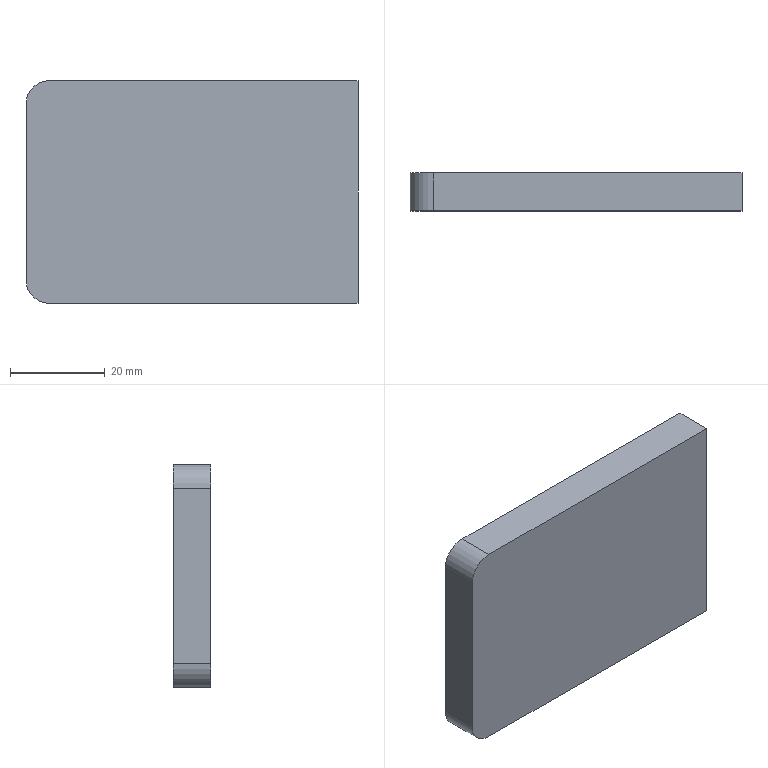Part | STEP file | 1 solid | 8 faces | box 70 x 8 x 47 mm | volume 26234 mm3 | plane 6 | cylinder 2 | commonest cylinder face diameters 10 x2
STEP:
#1=CARTESIAN_POINT('',(0.,0.,0.));
#2=DIRECTION('',(0.,0.,1.));
#3=DIRECTION('',(1.,0.,0.));
#4=AXIS2_PLACEMENT_3D('',#1,#2,#3);
#5=CARTESIAN_POINT('',(-247.863,95.5,183.951));
#6=VERTEX_POINT('',#5);
#7=CARTESIAN_POINT('',(-247.863,103.5,183.951));
#8=VERTEX_POINT('',#7);
#9=CARTESIAN_POINT('',(-247.863,103.5,183.951));
#10=DIRECTION('',(0.,1.,0.));
#11=VECTOR('',#10,1.);
#12=LINE('',#9,#11);
#13=CARTESIAN_POINT('',(-217.863,97.,183.951));
#14=DIRECTION('',(0.,0.,1.));
#15=DIRECTION('',(1.,0.,0.));
#16=AXIS2_PLACEMENT_3D('',#13,#14,#15);
#17=PLANE('',#16);
#18=CARTESIAN_POINT('',(-30.,6.5));
#19=DIRECTION('',(0.,1.));
#20=VECTOR('',#19,1.);
#21=LINE('',#18,#20);
#22=(GEOMETRIC_REPRESENTATION_CONTEXT(2)PARAMETRIC_REPRESENTATION_CONTEXT()REPRESENTATION_CONTEXT('',''));
#23=DEFINITIONAL_REPRESENTATION('',(#21),#22);
#24=PCURVE('',#17,#23);
#25=CARTESIAN_POINT('',(-247.863,69.939,178.951));
#26=DIRECTION('',(0.,1.,0.));
#27=DIRECTION('',(0.,0.,1.));
#28=AXIS2_PLACEMENT_3D('',#25,#26,#27);
#29=CYLINDRICAL_SURFACE('',#28,5.);
#30=CARTESIAN_POINT('',(6.283,33.561));
#31=DIRECTION('',(0.,1.));
#32=VECTOR('',#31,1.);
#33=LINE('',#30,#32);
#34=(GEOMETRIC_REPRESENTATION_CONTEXT(2)PARAMETRIC_REPRESENTATION_CONTEXT()REPRESENTATION_CONTEXT('',''));
#35=DEFINITIONAL_REPRESENTATION('',(#33),#34);
#36=PCURVE('',#29,#35);
#37=SURFACE_CURVE('',#12,(#24,#36),.PCURVE_S1.);
#38=EDGE_CURVE('',#6,#8,#37,.T.);
#39=ORIENTED_EDGE('',*,*,#38,.F.);
#40=CARTESIAN_POINT('',(-182.863,95.5,183.951));
#41=VERTEX_POINT('',#40);
#42=CARTESIAN_POINT('',(-217.863,95.5,183.951));
#43=DIRECTION('',(-1.,0.,0.));
#44=VECTOR('',#43,1.);
#45=LINE('',#42,#44);
#46=CARTESIAN_POINT('',(0.,-1.5));
#47=DIRECTION('',(-1.,0.));
#48=VECTOR('',#47,1.);
#49=LINE('',#46,#48);
#50=(GEOMETRIC_REPRESENTATION_CONTEXT(2)PARAMETRIC_REPRESENTATION_CONTEXT()REPRESENTATION_CONTEXT('',''));
#51=DEFINITIONAL_REPRESENTATION('',(#49),#50);
#52=PCURVE('',#17,#51);
#53=CARTESIAN_POINT('',(-217.863,95.5,136.951));
#54=DIRECTION('',(0.,-1.,0.));
#55=DIRECTION('',(0.,0.,-1.));
#56=AXIS2_PLACEMENT_3D('',#53,#54,#55);
#57=PLANE('',#56);
#58=CARTESIAN_POINT('',(-47.,0.));
#59=DIRECTION('',(0.,-1.));
#60=VECTOR('',#59,1.);
#61=LINE('',#58,#60);
#62=(GEOMETRIC_REPRESENTATION_CONTEXT(2)PARAMETRIC_REPRESENTATION_CONTEXT()REPRESENTATION_CONTEXT('',''));
#63=DEFINITIONAL_REPRESENTATION('',(#61),#62);
#64=PCURVE('',#57,#63);
#65=SURFACE_CURVE('',#45,(#52,#64),.PCURVE_S1.);
#66=EDGE_CURVE('',#41,#6,#65,.T.);
#67=ORIENTED_EDGE('',*,*,#66,.F.);
#68=CARTESIAN_POINT('',(-182.863,103.5,183.951));
#69=VERTEX_POINT('',#68);
#70=CARTESIAN_POINT('',(-182.863,97.,183.951));
#71=DIRECTION('',(0.,-1.,0.));
#72=VECTOR('',#71,1.);
#73=LINE('',#70,#72);
#74=CARTESIAN_POINT('',(35.,0.));
#75=DIRECTION('',(0.,-1.));
#76=VECTOR('',#75,1.);
#77=LINE('',#74,#76);
#78=(GEOMETRIC_REPRESENTATION_CONTEXT(2)PARAMETRIC_REPRESENTATION_CONTEXT()REPRESENTATION_CONTEXT('',''));
#79=DEFINITIONAL_REPRESENTATION('',(#77),#78);
#80=PCURVE('',#17,#79);
#81=CARTESIAN_POINT('',(-182.863,97.,136.951));
#82=DIRECTION('',(1.,0.,0.));
#83=DIRECTION('',(0.,0.,-1.));
#84=AXIS2_PLACEMENT_3D('',#81,#82,#83);
#85=PLANE('',#84);
#86=CARTESIAN_POINT('',(-47.,0.));
#87=DIRECTION('',(0.,-1.));
#88=VECTOR('',#87,1.);
#89=LINE('',#86,#88);
#90=(GEOMETRIC_REPRESENTATION_CONTEXT(2)PARAMETRIC_REPRESENTATION_CONTEXT()REPRESENTATION_CONTEXT('',''));
#91=DEFINITIONAL_REPRESENTATION('',(#89),#90);
#92=PCURVE('',#85,#91);
#93=SURFACE_CURVE('',#73,(#80,#92),.PCURVE_S1.);
#94=EDGE_CURVE('',#69,#41,#93,.T.);
#95=ORIENTED_EDGE('',*,*,#94,.F.);
#96=CARTESIAN_POINT('',(-217.863,103.5,183.951));
#97=DIRECTION('',(1.,0.,0.));
#98=VECTOR('',#97,1.);
#99=LINE('',#96,#98);
#100=CARTESIAN_POINT('',(0.,6.5));
#101=DIRECTION('',(1.,0.));
#102=VECTOR('',#101,1.);
#103=LINE('',#100,#102);
#104=(GEOMETRIC_REPRESENTATION_CONTEXT(2)PARAMETRIC_REPRESENTATION_CONTEXT()REPRESENTATION_CONTEXT('',''));
#105=DEFINITIONAL_REPRESENTATION('',(#103),#104);
#106=PCURVE('',#17,#105);
#107=CARTESIAN_POINT('',(-217.863,103.5,136.951));
#108=DIRECTION('',(0.,1.,0.));
#109=DIRECTION('',(0.,0.,1.));
#110=AXIS2_PLACEMENT_3D('',#107,#108,#109);
#111=PLANE('',#110);
#112=CARTESIAN_POINT('',(47.,0.));
#113=DIRECTION('',(0.,1.));
#114=VECTOR('',#113,1.);
#115=LINE('',#112,#114);
#116=(GEOMETRIC_REPRESENTATION_CONTEXT(2)PARAMETRIC_REPRESENTATION_CONTEXT()REPRESENTATION_CONTEXT('',''));
#117=DEFINITIONAL_REPRESENTATION('',(#115),#116);
#118=PCURVE('',#111,#117);
#119=SURFACE_CURVE('',#99,(#106,#118),.PCURVE_S1.);
#120=EDGE_CURVE('',#8,#69,#119,.T.);
#121=ORIENTED_EDGE('',*,*,#120,.F.);
#122=EDGE_LOOP('',(#39,#67,#95,#121));
#123=FACE_BOUND('',#122,.T.);
#124=ADVANCED_FACE('',(#123),#17,.T.);
#125=CARTESIAN_POINT('',(-247.863,95.5,136.951));
#126=VERTEX_POINT('',#125);
#127=CARTESIAN_POINT('',(-252.863,95.5,141.951));
#128=VERTEX_POINT('',#127);
#129=CARTESIAN_POINT('',(-247.863,95.5,141.951));
#130=DIRECTION('',(0.,1.,0.));
#131=DIRECTION('',(0.,0.,-1.));
#132=AXIS2_PLACEMENT_3D('',#129,#130,#131);
#133=CIRCLE('',#132,5.);
#134=CARTESIAN_POINT('',(0.,-30.));
#135=CARTESIAN_POINT('',(0.,-38.66));
#136=CARTESIAN_POINT('',(-7.5,-34.33));
#137=CARTESIAN_POINT('',(-15.,-30.));
#138=CARTESIAN_POINT('',(-7.5,-25.67));
#139=CARTESIAN_POINT('',(0.,-21.34));
#140=CARTESIAN_POINT('',(0.,-30.));
#141=(BOUNDED_CURVE()B_SPLINE_CURVE(2,(#134,#135,#136,#137,#138,#139,#140),.UNSPECIFIED.,.T.,.F.)B_SPLINE_CURVE_WITH_KNOTS((1,2,2,2,2,1),(-2.094,0.,2.094,4.189,6.283,8.378),.UNSPECIFIED.)CURVE()GEOMETRIC_REPRESENTATION_ITEM()RATIONAL_B_SPLINE_CURVE((1.,0.5,1.,0.5,1.,0.5,1.))REPRESENTATION_ITEM(''));
#142=(GEOMETRIC_REPRESENTATION_CONTEXT(2)PARAMETRIC_REPRESENTATION_CONTEXT()REPRESENTATION_CONTEXT('',''));
#143=DEFINITIONAL_REPRESENTATION('',(#141),#142);
#144=PCURVE('',#57,#143);
#145=CARTESIAN_POINT('',(-247.863,80.5,141.951));
#146=DIRECTION('',(0.,-1.,0.));
#147=DIRECTION('',(0.,0.,-1.));
#148=AXIS2_PLACEMENT_3D('',#145,#146,#147);
#149=CYLINDRICAL_SURFACE('',#148,5.);
#150=CARTESIAN_POINT('',(6.283,-15.));
#151=DIRECTION('',(-1.,0.));
#152=VECTOR('',#151,1.);
#153=LINE('',#150,#152);
#154=(GEOMETRIC_REPRESENTATION_CONTEXT(2)PARAMETRIC_REPRESENTATION_CONTEXT()REPRESENTATION_CONTEXT('',''));
#155=DEFINITIONAL_REPRESENTATION('',(#153),#154);
#156=PCURVE('',#149,#155);
#157=SURFACE_CURVE('',#133,(#144,#156),.PCURVE_S1.);
#158=EDGE_CURVE('',#126,#128,#157,.T.);
#159=ORIENTED_EDGE('',*,*,#158,.F.);
#160=CARTESIAN_POINT('',(-182.863,95.5,136.951));
#161=VERTEX_POINT('',#160);
#162=CARTESIAN_POINT('',(-217.863,95.5,136.951));
#163=DIRECTION('',(1.,0.,0.));
#164=VECTOR('',#163,1.);
#165=LINE('',#162,#164);
#166=CARTESIAN_POINT('',(0.,0.));
#167=DIRECTION('',(0.,1.));
#168=VECTOR('',#167,1.);
#169=LINE('',#166,#168);
#170=(GEOMETRIC_REPRESENTATION_CONTEXT(2)PARAMETRIC_REPRESENTATION_CONTEXT()REPRESENTATION_CONTEXT('',''));
#171=DEFINITIONAL_REPRESENTATION('',(#169),#170);
#172=PCURVE('',#57,#171);
#173=CARTESIAN_POINT('',(-217.863,97.,136.951));
#174=DIRECTION('',(0.,0.,-1.));
#175=DIRECTION('',(-1.,0.,0.));
#176=AXIS2_PLACEMENT_3D('',#173,#174,#175);
#177=PLANE('',#176);
#178=CARTESIAN_POINT('',(0.,-1.5));
#179=DIRECTION('',(-1.,0.));
#180=VECTOR('',#179,1.);
#181=LINE('',#178,#180);
#182=(GEOMETRIC_REPRESENTATION_CONTEXT(2)PARAMETRIC_REPRESENTATION_CONTEXT()REPRESENTATION_CONTEXT('',''));
#183=DEFINITIONAL_REPRESENTATION('',(#181),#182);
#184=PCURVE('',#177,#183);
#185=SURFACE_CURVE('',#165,(#172,#184),.PCURVE_S1.);
#186=EDGE_CURVE('',#126,#161,#185,.T.);
#187=ORIENTED_EDGE('',*,*,#186,.T.);
#188=CARTESIAN_POINT('',(-182.863,95.5,136.951));
#189=DIRECTION('',(0.,0.,1.));
#190=VECTOR('',#189,1.);
#191=LINE('',#188,#190);
#192=CARTESIAN_POINT('',(0.,35.));
#193=DIRECTION('',(-1.,0.));
#194=VECTOR('',#193,1.);
#195=LINE('',#192,#194);
#196=(GEOMETRIC_REPRESENTATION_CONTEXT(2)PARAMETRIC_REPRESENTATION_CONTEXT()REPRESENTATION_CONTEXT('',''));
#197=DEFINITIONAL_REPRESENTATION('',(#195),#196);
#198=PCURVE('',#57,#197);
#199=CARTESIAN_POINT('',(0.,-1.5));
#200=DIRECTION('',(-1.,0.));
#201=VECTOR('',#200,1.);
#202=LINE('',#199,#201);
#203=(GEOMETRIC_REPRESENTATION_CONTEXT(2)PARAMETRIC_REPRESENTATION_CONTEXT()REPRESENTATION_CONTEXT('',''));
#204=DEFINITIONAL_REPRESENTATION('',(#202),#203);
#205=PCURVE('',#85,#204);
#206=SURFACE_CURVE('',#191,(#198,#205),.PCURVE_S1.);
#207=EDGE_CURVE('',#161,#41,#206,.T.);
#208=ORIENTED_EDGE('',*,*,#207,.T.);
#209=ORIENTED_EDGE('',*,*,#66,.T.);
#210=CARTESIAN_POINT('',(-252.863,95.5,178.951));
#211=VERTEX_POINT('',#210);
#212=CARTESIAN_POINT('',(-247.863,95.5,178.951));
#213=DIRECTION('',(0.,1.,0.));
#214=DIRECTION('',(0.,0.,-1.));
#215=AXIS2_PLACEMENT_3D('',#212,#213,#214);
#216=CIRCLE('',#215,5.);
#217=CARTESIAN_POINT('',(-37.,-30.));
#218=CARTESIAN_POINT('',(-37.,-38.66));
#219=CARTESIAN_POINT('',(-44.5,-34.33));
#220=CARTESIAN_POINT('',(-52.,-30.));
#221=CARTESIAN_POINT('',(-44.5,-25.67));
#222=CARTESIAN_POINT('',(-37.,-21.34));
#223=CARTESIAN_POINT('',(-37.,-30.));
#224=(BOUNDED_CURVE()B_SPLINE_CURVE(2,(#217,#218,#219,#220,#221,#222,#223),.UNSPECIFIED.,.T.,.F.)B_SPLINE_CURVE_WITH_KNOTS((1,2,2,2,2,1),(-2.094,0.,2.094,4.189,6.283,8.378),.UNSPECIFIED.)CURVE()GEOMETRIC_REPRESENTATION_ITEM()RATIONAL_B_SPLINE_CURVE((1.,0.5,1.,0.5,1.,0.5,1.))REPRESENTATION_ITEM(''));
#225=(GEOMETRIC_REPRESENTATION_CONTEXT(2)PARAMETRIC_REPRESENTATION_CONTEXT()REPRESENTATION_CONTEXT('',''));
#226=DEFINITIONAL_REPRESENTATION('',(#224),#225);
#227=PCURVE('',#57,#226);
#228=CARTESIAN_POINT('',(3.142,25.561));
#229=DIRECTION('',(1.,0.));
#230=VECTOR('',#229,1.);
#231=LINE('',#228,#230);
#232=(GEOMETRIC_REPRESENTATION_CONTEXT(2)PARAMETRIC_REPRESENTATION_CONTEXT()REPRESENTATION_CONTEXT('',''));
#233=DEFINITIONAL_REPRESENTATION('',(#231),#232);
#234=PCURVE('',#29,#233);
#235=SURFACE_CURVE('',#216,(#227,#234),.PCURVE_S1.);
#236=EDGE_CURVE('',#211,#6,#235,.T.);
#237=ORIENTED_EDGE('',*,*,#236,.F.);
#238=CARTESIAN_POINT('',(-252.863,95.5,136.951));
#239=DIRECTION('',(0.,0.,1.));
#240=VECTOR('',#239,1.);
#241=LINE('',#238,#240);
#242=CARTESIAN_POINT('',(0.,-35.));
#243=DIRECTION('',(-1.,0.));
#244=VECTOR('',#243,1.);
#245=LINE('',#242,#244);
#246=(GEOMETRIC_REPRESENTATION_CONTEXT(2)PARAMETRIC_REPRESENTATION_CONTEXT()REPRESENTATION_CONTEXT('',''));
#247=DEFINITIONAL_REPRESENTATION('',(#245),#246);
#248=PCURVE('',#57,#247);
#249=CARTESIAN_POINT('',(-252.863,97.,136.951));
#250=DIRECTION('',(-1.,0.,0.));
#251=DIRECTION('',(0.,0.,1.));
#252=AXIS2_PLACEMENT_3D('',#249,#250,#251);
#253=PLANE('',#252);
#254=CARTESIAN_POINT('',(0.,-1.5));
#255=DIRECTION('',(1.,0.));
#256=VECTOR('',#255,1.);
#257=LINE('',#254,#256);
#258=(GEOMETRIC_REPRESENTATION_CONTEXT(2)PARAMETRIC_REPRESENTATION_CONTEXT()REPRESENTATION_CONTEXT('',''));
#259=DEFINITIONAL_REPRESENTATION('',(#257),#258);
#260=PCURVE('',#253,#259);
#261=SURFACE_CURVE('',#241,(#248,#260),.PCURVE_S1.);
#262=EDGE_CURVE('',#128,#211,#261,.T.);
#263=ORIENTED_EDGE('',*,*,#262,.F.);
#264=EDGE_LOOP('',(#159,#187,#208,#209,#237,#263));
#265=FACE_BOUND('',#264,.T.);
#266=ADVANCED_FACE('',(#265),#57,.T.);
#267=CARTESIAN_POINT('',(-252.863,103.5,141.951));
#268=VERTEX_POINT('',#267);
#269=CARTESIAN_POINT('',(-252.863,80.5,141.951));
#270=DIRECTION('',(0.,1.,0.));
#271=VECTOR('',#270,1.);
#272=LINE('',#269,#271);
#273=CARTESIAN_POINT('',(5.,-16.5));
#274=DIRECTION('',(0.,1.));
#275=VECTOR('',#274,1.);
#276=LINE('',#273,#275);
#277=(GEOMETRIC_REPRESENTATION_CONTEXT(2)PARAMETRIC_REPRESENTATION_CONTEXT()REPRESENTATION_CONTEXT('',''));
#278=DEFINITIONAL_REPRESENTATION('',(#276),#277);
#279=PCURVE('',#253,#278);
#280=CARTESIAN_POINT('',(4.712,0.));
#281=DIRECTION('',(0.,-1.));
#282=VECTOR('',#281,1.);
#283=LINE('',#280,#282);
#284=(GEOMETRIC_REPRESENTATION_CONTEXT(2)PARAMETRIC_REPRESENTATION_CONTEXT()REPRESENTATION_CONTEXT('',''));
#285=DEFINITIONAL_REPRESENTATION('',(#283),#284);
#286=PCURVE('',#149,#285);
#287=SURFACE_CURVE('',#272,(#279,#286),.PCURVE_S1.);
#288=EDGE_CURVE('',#128,#268,#287,.T.);
#289=ORIENTED_EDGE('',*,*,#288,.F.);
#290=ORIENTED_EDGE('',*,*,#262,.T.);
#291=CARTESIAN_POINT('',(-252.863,103.5,178.951));
#292=VERTEX_POINT('',#291);
#293=CARTESIAN_POINT('',(-252.863,90.5,178.951));
#294=DIRECTION('',(0.,-1.,0.));
#295=VECTOR('',#294,1.);
#296=LINE('',#293,#295);
#297=CARTESIAN_POINT('',(42.,-6.5));
#298=DIRECTION('',(0.,-1.));
#299=VECTOR('',#298,1.);
#300=LINE('',#297,#299);
#301=(GEOMETRIC_REPRESENTATION_CONTEXT(2)PARAMETRIC_REPRESENTATION_CONTEXT()REPRESENTATION_CONTEXT('',''));
#302=DEFINITIONAL_REPRESENTATION('',(#300),#301);
#303=PCURVE('',#253,#302);
#304=CARTESIAN_POINT('',(4.712,20.561));
#305=DIRECTION('',(0.,-1.));
#306=VECTOR('',#305,1.);
#307=LINE('',#304,#306);
#308=(GEOMETRIC_REPRESENTATION_CONTEXT(2)PARAMETRIC_REPRESENTATION_CONTEXT()REPRESENTATION_CONTEXT('',''));
#309=DEFINITIONAL_REPRESENTATION('',(#307),#308);
#310=PCURVE('',#29,#309);
#311=SURFACE_CURVE('',#296,(#303,#310),.PCURVE_S1.);
#312=EDGE_CURVE('',#292,#211,#311,.T.);
#313=ORIENTED_EDGE('',*,*,#312,.F.);
#314=CARTESIAN_POINT('',(-252.863,103.5,136.951));
#315=DIRECTION('',(0.,0.,1.));
#316=VECTOR('',#315,1.);
#317=LINE('',#314,#316);
#318=CARTESIAN_POINT('',(0.,6.5));
#319=DIRECTION('',(1.,0.));
#320=VECTOR('',#319,1.);
#321=LINE('',#318,#320);
#322=(GEOMETRIC_REPRESENTATION_CONTEXT(2)PARAMETRIC_REPRESENTATION_CONTEXT()REPRESENTATION_CONTEXT('',''));
#323=DEFINITIONAL_REPRESENTATION('',(#321),#322);
#324=PCURVE('',#253,#323);
#325=CARTESIAN_POINT('',(0.,-35.));
#326=DIRECTION('',(1.,0.));
#327=VECTOR('',#326,1.);
#328=LINE('',#325,#327);
#329=(GEOMETRIC_REPRESENTATION_CONTEXT(2)PARAMETRIC_REPRESENTATION_CONTEXT()REPRESENTATION_CONTEXT('',''));
#330=DEFINITIONAL_REPRESENTATION('',(#328),#329);
#331=PCURVE('',#111,#330);
#332=SURFACE_CURVE('',#317,(#324,#331),.PCURVE_S1.);
#333=EDGE_CURVE('',#268,#292,#332,.T.);
#334=ORIENTED_EDGE('',*,*,#333,.F.);
#335=EDGE_LOOP('',(#289,#290,#313,#334));
#336=FACE_BOUND('',#335,.T.);
#337=ADVANCED_FACE('',(#336),#253,.T.);
#338=CARTESIAN_POINT('',(-247.863,103.5,178.951));
#339=DIRECTION('',(0.,-1.,0.));
#340=DIRECTION('',(0.,0.,-1.));
#341=AXIS2_PLACEMENT_3D('',#338,#339,#340);
#342=CIRCLE('',#341,5.);
#343=CARTESIAN_POINT('',(37.,-30.));
#344=CARTESIAN_POINT('',(37.,-21.34));
#345=CARTESIAN_POINT('',(44.5,-25.67));
#346=CARTESIAN_POINT('',(52.,-30.));
#347=CARTESIAN_POINT('',(44.5,-34.33));
#348=CARTESIAN_POINT('',(37.,-38.66));
#349=CARTESIAN_POINT('',(37.,-30.));
#350=(BOUNDED_CURVE()B_SPLINE_CURVE(2,(#343,#344,#345,#346,#347,#348,#349),.UNSPECIFIED.,.T.,.F.)B_SPLINE_CURVE_WITH_KNOTS((1,2,2,2,2,1),(-2.094,0.,2.094,4.189,6.283,8.378),.UNSPECIFIED.)CURVE()GEOMETRIC_REPRESENTATION_ITEM()RATIONAL_B_SPLINE_CURVE((1.,0.5,1.,0.5,1.,0.5,1.))REPRESENTATION_ITEM(''));
#351=(GEOMETRIC_REPRESENTATION_CONTEXT(2)PARAMETRIC_REPRESENTATION_CONTEXT()REPRESENTATION_CONTEXT('',''));
#352=DEFINITIONAL_REPRESENTATION('',(#350),#351);
#353=PCURVE('',#111,#352);
#354=CARTESIAN_POINT('',(9.425,33.561));
#355=DIRECTION('',(-1.,0.));
#356=VECTOR('',#355,1.);
#357=LINE('',#354,#356);
#358=(GEOMETRIC_REPRESENTATION_CONTEXT(2)PARAMETRIC_REPRESENTATION_CONTEXT()REPRESENTATION_CONTEXT('',''));
#359=DEFINITIONAL_REPRESENTATION('',(#357),#358);
#360=PCURVE('',#29,#359);
#361=SURFACE_CURVE('',#342,(#353,#360),.PCURVE_S1.);
#362=EDGE_CURVE('',#8,#292,#361,.T.);
#363=ORIENTED_EDGE('',*,*,#362,.F.);
#364=ORIENTED_EDGE('',*,*,#120,.T.);
#365=CARTESIAN_POINT('',(-182.863,103.5,136.951));
#366=VERTEX_POINT('',#365);
#367=CARTESIAN_POINT('',(-182.863,103.5,136.951));
#368=DIRECTION('',(0.,0.,1.));
#369=VECTOR('',#368,1.);
#370=LINE('',#367,#369);
#371=CARTESIAN_POINT('',(0.,35.));
#372=DIRECTION('',(1.,0.));
#373=VECTOR('',#372,1.);
#374=LINE('',#371,#373);
#375=(GEOMETRIC_REPRESENTATION_CONTEXT(2)PARAMETRIC_REPRESENTATION_CONTEXT()REPRESENTATION_CONTEXT('',''));
#376=DEFINITIONAL_REPRESENTATION('',(#374),#375);
#377=PCURVE('',#111,#376);
#378=CARTESIAN_POINT('',(0.,6.5));
#379=DIRECTION('',(-1.,0.));
#380=VECTOR('',#379,1.);
#381=LINE('',#378,#380);
#382=(GEOMETRIC_REPRESENTATION_CONTEXT(2)PARAMETRIC_REPRESENTATION_CONTEXT()REPRESENTATION_CONTEXT('',''));
#383=DEFINITIONAL_REPRESENTATION('',(#381),#382);
#384=PCURVE('',#85,#383);
#385=SURFACE_CURVE('',#370,(#377,#384),.PCURVE_S1.);
#386=EDGE_CURVE('',#366,#69,#385,.T.);
#387=ORIENTED_EDGE('',*,*,#386,.F.);
#388=CARTESIAN_POINT('',(-247.863,103.5,136.951));
#389=VERTEX_POINT('',#388);
#390=CARTESIAN_POINT('',(-217.863,103.5,136.951));
#391=DIRECTION('',(-1.,0.,0.));
#392=VECTOR('',#391,1.);
#393=LINE('',#390,#392);
#394=CARTESIAN_POINT('',(0.,0.));
#395=DIRECTION('',(0.,-1.));
#396=VECTOR('',#395,1.);
#397=LINE('',#394,#396);
#398=(GEOMETRIC_REPRESENTATION_CONTEXT(2)PARAMETRIC_REPRESENTATION_CONTEXT()REPRESENTATION_CONTEXT('',''));
#399=DEFINITIONAL_REPRESENTATION('',(#397),#398);
#400=PCURVE('',#111,#399);
#401=CARTESIAN_POINT('',(0.,6.5));
#402=DIRECTION('',(1.,0.));
#403=VECTOR('',#402,1.);
#404=LINE('',#401,#403);
#405=(GEOMETRIC_REPRESENTATION_CONTEXT(2)PARAMETRIC_REPRESENTATION_CONTEXT()REPRESENTATION_CONTEXT('',''));
#406=DEFINITIONAL_REPRESENTATION('',(#404),#405);
#407=PCURVE('',#177,#406);
#408=SURFACE_CURVE('',#393,(#400,#407),.PCURVE_S1.);
#409=EDGE_CURVE('',#366,#389,#408,.T.);
#410=ORIENTED_EDGE('',*,*,#409,.T.);
#411=CARTESIAN_POINT('',(-247.863,103.5,141.951));
#412=DIRECTION('',(0.,-1.,0.));
#413=DIRECTION('',(0.,0.,-1.));
#414=AXIS2_PLACEMENT_3D('',#411,#412,#413);
#415=CIRCLE('',#414,5.);
#416=CARTESIAN_POINT('',(0.,-30.));
#417=CARTESIAN_POINT('',(0.,-21.34));
#418=CARTESIAN_POINT('',(7.5,-25.67));
#419=CARTESIAN_POINT('',(15.,-30.));
#420=CARTESIAN_POINT('',(7.5,-34.33));
#421=CARTESIAN_POINT('',(0.,-38.66));
#422=CARTESIAN_POINT('',(0.,-30.));
#423=(BOUNDED_CURVE()B_SPLINE_CURVE(2,(#416,#417,#418,#419,#420,#421,#422),.UNSPECIFIED.,.T.,.F.)B_SPLINE_CURVE_WITH_KNOTS((1,2,2,2,2,1),(-2.094,0.,2.094,4.189,6.283,8.378),.UNSPECIFIED.)CURVE()GEOMETRIC_REPRESENTATION_ITEM()RATIONAL_B_SPLINE_CURVE((1.,0.5,1.,0.5,1.,0.5,1.))REPRESENTATION_ITEM(''));
#424=(GEOMETRIC_REPRESENTATION_CONTEXT(2)PARAMETRIC_REPRESENTATION_CONTEXT()REPRESENTATION_CONTEXT('',''));
#425=DEFINITIONAL_REPRESENTATION('',(#423),#424);
#426=PCURVE('',#111,#425);
#427=CARTESIAN_POINT('',(0.,-23.));
#428=DIRECTION('',(1.,0.));
#429=VECTOR('',#428,1.);
#430=LINE('',#427,#429);
#431=(GEOMETRIC_REPRESENTATION_CONTEXT(2)PARAMETRIC_REPRESENTATION_CONTEXT()REPRESENTATION_CONTEXT('',''));
#432=DEFINITIONAL_REPRESENTATION('',(#430),#431);
#433=PCURVE('',#149,#432);
#434=SURFACE_CURVE('',#415,(#426,#433),.PCURVE_S1.);
#435=EDGE_CURVE('',#268,#389,#434,.T.);
#436=ORIENTED_EDGE('',*,*,#435,.F.);
#437=ORIENTED_EDGE('',*,*,#333,.T.);
#438=EDGE_LOOP('',(#363,#364,#387,#410,#436,#437));
#439=FACE_BOUND('',#438,.T.);
#440=ADVANCED_FACE('',(#439),#111,.T.);
#441=CARTESIAN_POINT('',(-247.863,69.939,136.951));
#442=DIRECTION('',(0.,-1.,0.));
#443=VECTOR('',#442,1.);
#444=LINE('',#441,#443);
#445=CARTESIAN_POINT('',(30.,-27.061));
#446=DIRECTION('',(0.,-1.));
#447=VECTOR('',#446,1.);
#448=LINE('',#445,#447);
#449=(GEOMETRIC_REPRESENTATION_CONTEXT(2)PARAMETRIC_REPRESENTATION_CONTEXT()REPRESENTATION_CONTEXT('',''));
#450=DEFINITIONAL_REPRESENTATION('',(#448),#449);
#451=PCURVE('',#177,#450);
#452=CARTESIAN_POINT('',(6.283,10.561));
#453=DIRECTION('',(0.,1.));
#454=VECTOR('',#453,1.);
#455=LINE('',#452,#454);
#456=(GEOMETRIC_REPRESENTATION_CONTEXT(2)PARAMETRIC_REPRESENTATION_CONTEXT()REPRESENTATION_CONTEXT('',''));
#457=DEFINITIONAL_REPRESENTATION('',(#455),#456);
#458=PCURVE('',#149,#457);
#459=SURFACE_CURVE('',#444,(#451,#458),.PCURVE_S1.);
#460=EDGE_CURVE('',#389,#126,#459,.T.);
#461=ORIENTED_EDGE('',*,*,#460,.F.);
#462=ORIENTED_EDGE('',*,*,#409,.F.);
#463=CARTESIAN_POINT('',(-182.863,97.,136.951));
#464=DIRECTION('',(0.,1.,0.));
#465=VECTOR('',#464,1.);
#466=LINE('',#463,#465);
#467=CARTESIAN_POINT('',(-35.,0.));
#468=DIRECTION('',(0.,1.));
#469=VECTOR('',#468,1.);
#470=LINE('',#467,#469);
#471=(GEOMETRIC_REPRESENTATION_CONTEXT(2)PARAMETRIC_REPRESENTATION_CONTEXT()REPRESENTATION_CONTEXT('',''));
#472=DEFINITIONAL_REPRESENTATION('',(#470),#471);
#473=PCURVE('',#177,#472);
#474=CARTESIAN_POINT('',(0.,0.));
#475=DIRECTION('',(0.,1.));
#476=VECTOR('',#475,1.);
#477=LINE('',#474,#476);
#478=(GEOMETRIC_REPRESENTATION_CONTEXT(2)PARAMETRIC_REPRESENTATION_CONTEXT()REPRESENTATION_CONTEXT('',''));
#479=DEFINITIONAL_REPRESENTATION('',(#477),#478);
#480=PCURVE('',#85,#479);
#481=SURFACE_CURVE('',#466,(#473,#480),.PCURVE_S1.);
#482=EDGE_CURVE('',#161,#366,#481,.T.);
#483=ORIENTED_EDGE('',*,*,#482,.F.);
#484=ORIENTED_EDGE('',*,*,#186,.F.);
#485=EDGE_LOOP('',(#461,#462,#483,#484));
#486=FACE_BOUND('',#485,.T.);
#487=ADVANCED_FACE('',(#486),#177,.T.);
#488=ORIENTED_EDGE('',*,*,#482,.T.);
#489=ORIENTED_EDGE('',*,*,#386,.T.);
#490=ORIENTED_EDGE('',*,*,#94,.T.);
#491=ORIENTED_EDGE('',*,*,#207,.F.);
#492=EDGE_LOOP('',(#488,#489,#490,#491));
#493=FACE_BOUND('',#492,.T.);
#494=ADVANCED_FACE('',(#493),#85,.T.);
#495=ORIENTED_EDGE('',*,*,#158,.T.);
#496=ORIENTED_EDGE('',*,*,#288,.T.);
#497=ORIENTED_EDGE('',*,*,#435,.T.);
#498=ORIENTED_EDGE('',*,*,#460,.T.);
#499=EDGE_LOOP('',(#495,#496,#497,#498));
#500=FACE_BOUND('',#499,.T.);
#501=ADVANCED_FACE('',(#500),#149,.T.);
#502=ORIENTED_EDGE('',*,*,#236,.T.);
#503=ORIENTED_EDGE('',*,*,#38,.T.);
#504=ORIENTED_EDGE('',*,*,#362,.T.);
#505=ORIENTED_EDGE('',*,*,#312,.T.);
#506=EDGE_LOOP('',(#502,#503,#504,#505));
#507=FACE_BOUND('',#506,.T.);
#508=ADVANCED_FACE('',(#507),#29,.T.);
#509=CLOSED_SHELL('',(#124,#266,#337,#440,#487,#494,#501,#508));
#510=MANIFOLD_SOLID_BREP('',#509);
#511=(LENGTH_UNIT()NAMED_UNIT(*)SI_UNIT(.MILLI.,.METRE.));
#512=UNCERTAINTY_MEASURE_WITH_UNIT(LENGTH_MEASURE(0.0000001),#511,'','');
#513=(NAMED_UNIT(*)PLANE_ANGLE_UNIT()SI_UNIT($,.RADIAN.));
#514=(NAMED_UNIT(*)SI_UNIT($,.STERADIAN.)SOLID_ANGLE_UNIT());
#515=(GEOMETRIC_REPRESENTATION_CONTEXT(3)GLOBAL_UNCERTAINTY_ASSIGNED_CONTEXT((#512))GLOBAL_UNIT_ASSIGNED_CONTEXT((#511,#513,#514))REPRESENTATION_CONTEXT('',''));
#516=ADVANCED_BREP_SHAPE_REPRESENTATION('',(#4,#510),#515);